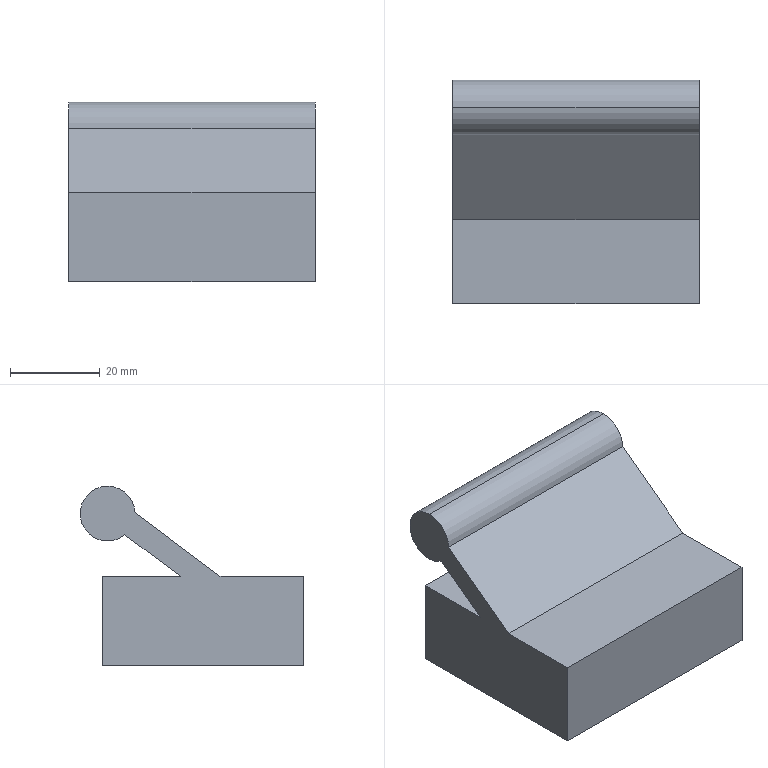Part | STEP file | Power switch 1 | 1 solid | 12 faces | box 55 x 49.883 x 40.112 mm | volume 61552 mm3 | plane 9 | cylinder 3 | commonest cylinder face diameters 12.241 x3
STEP:
#1=CARTESIAN_POINT('',(0.,0.,0.));
#2=DIRECTION('',(0.,0.,1.));
#3=DIRECTION('',(1.,0.,0.));
#4=AXIS2_PLACEMENT_3D('',#1,#2,#3);
#5=CARTESIAN_POINT('',(-27.5,21.263,27.872));
#6=VERTEX_POINT('',#5);
#7=CARTESIAN_POINT('',(-27.5,21.263,40.112));
#8=VERTEX_POINT('',#7);
#9=CARTESIAN_POINT('',(-27.5,21.263,33.992));
#10=DIRECTION('',(1.,0.,0.));
#11=DIRECTION('',(0.,0.,-1.));
#12=AXIS2_PLACEMENT_3D('',#9,#10,#11);
#13=CIRCLE('',#12,6.12);
#14=CARTESIAN_POINT('',(-27.5,21.263,33.992));
#15=DIRECTION('',(1.,0.,0.));
#16=DIRECTION('',(0.,0.,-1.));
#17=AXIS2_PLACEMENT_3D('',#14,#15,#16);
#18=CYLINDRICAL_SURFACE('',#17,6.12);
#19=CARTESIAN_POINT('',(0.,0.));
#20=DIRECTION('',(1.,0.));
#21=VECTOR('',#20,1.);
#22=LINE('',#19,#21);
#23=(GEOMETRIC_REPRESENTATION_CONTEXT(2)PARAMETRIC_REPRESENTATION_CONTEXT()REPRESENTATION_CONTEXT('',''));
#24=DEFINITIONAL_REPRESENTATION('',(#22),#23);
#25=PCURVE('',#18,#24);
#26=CARTESIAN_POINT('',(-27.5,22.5,20.));
#27=DIRECTION('',(1.,0.,0.));
#28=DIRECTION('',(0.,1.,0.));
#29=AXIS2_PLACEMENT_3D('',#26,#27,#28);
#30=PLANE('',#29);
#31=CARTESIAN_POINT('',(-1.237,13.992));
#32=DIRECTION('',(0.,-1.));
#33=AXIS2_PLACEMENT_2D('',#31,#32);
#34=CIRCLE('',#33,6.12);
#35=(GEOMETRIC_REPRESENTATION_CONTEXT(2)PARAMETRIC_REPRESENTATION_CONTEXT()REPRESENTATION_CONTEXT('',''));
#36=DEFINITIONAL_REPRESENTATION('',(#34),#35);
#37=PCURVE('',#30,#36);
#38=SURFACE_CURVE('',#13,(#25,#37),.PCURVE_S1.);
#39=EDGE_CURVE('',#6,#8,#38,.T.);
#40=ORIENTED_EDGE('',*,*,#39,.T.);
#41=CARTESIAN_POINT('',(27.5,21.263,40.112));
#42=VERTEX_POINT('',#41);
#43=CARTESIAN_POINT('',(-27.5,21.263,40.112));
#44=DIRECTION('',(1.,0.,0.));
#45=VECTOR('',#44,1.);
#46=LINE('',#43,#45);
#47=CARTESIAN_POINT('',(3.142,0.));
#48=DIRECTION('',(0.,1.));
#49=VECTOR('',#48,1.);
#50=LINE('',#47,#49);
#51=(GEOMETRIC_REPRESENTATION_CONTEXT(2)PARAMETRIC_REPRESENTATION_CONTEXT()REPRESENTATION_CONTEXT('',''));
#52=DEFINITIONAL_REPRESENTATION('',(#50),#51);
#53=PCURVE('',#18,#52);
#54=CARTESIAN_POINT('',(-27.5,21.263,33.992));
#55=DIRECTION('',(1.,0.,0.));
#56=DIRECTION('',(0.,0.,-1.));
#57=AXIS2_PLACEMENT_3D('',#54,#55,#56);
#58=CYLINDRICAL_SURFACE('',#57,6.12);
#59=CARTESIAN_POINT('',(3.142,0.));
#60=DIRECTION('',(0.,1.));
#61=VECTOR('',#60,1.);
#62=LINE('',#59,#61);
#63=(GEOMETRIC_REPRESENTATION_CONTEXT(2)PARAMETRIC_REPRESENTATION_CONTEXT()REPRESENTATION_CONTEXT('',''));
#64=DEFINITIONAL_REPRESENTATION('',(#62),#63);
#65=PCURVE('',#58,#64);
#66=SURFACE_CURVE('',#46,(#53,#65),.PCURVE_S1.);
#67=EDGE_CURVE('',#8,#42,#66,.T.);
#68=ORIENTED_EDGE('',*,*,#67,.T.);
#69=CARTESIAN_POINT('',(27.5,21.263,27.872));
#70=VERTEX_POINT('',#69);
#71=CARTESIAN_POINT('',(27.5,21.263,33.992));
#72=DIRECTION('',(-1.,0.,0.));
#73=DIRECTION('',(0.,0.,-1.));
#74=AXIS2_PLACEMENT_3D('',#71,#72,#73);
#75=CIRCLE('',#74,6.12);
#76=CARTESIAN_POINT('',(6.283,55.));
#77=DIRECTION('',(-1.,0.));
#78=VECTOR('',#77,1.);
#79=LINE('',#76,#78);
#80=(GEOMETRIC_REPRESENTATION_CONTEXT(2)PARAMETRIC_REPRESENTATION_CONTEXT()REPRESENTATION_CONTEXT('',''));
#81=DEFINITIONAL_REPRESENTATION('',(#79),#80);
#82=PCURVE('',#18,#81);
#83=CARTESIAN_POINT('',(27.5,22.5,20.));
#84=DIRECTION('',(-1.,0.,0.));
#85=DIRECTION('',(0.,-1.,0.));
#86=AXIS2_PLACEMENT_3D('',#83,#84,#85);
#87=PLANE('',#86);
#88=CARTESIAN_POINT('',(1.237,13.992));
#89=DIRECTION('',(0.,-1.));
#90=AXIS2_PLACEMENT_2D('',#88,#89);
#91=CIRCLE('',#90,6.12);
#92=(GEOMETRIC_REPRESENTATION_CONTEXT(2)PARAMETRIC_REPRESENTATION_CONTEXT()REPRESENTATION_CONTEXT('',''));
#93=DEFINITIONAL_REPRESENTATION('',(#91),#92);
#94=PCURVE('',#87,#93);
#95=SURFACE_CURVE('',#75,(#82,#94),.PCURVE_S1.);
#96=EDGE_CURVE('',#42,#70,#95,.T.);
#97=ORIENTED_EDGE('',*,*,#96,.T.);
#98=CARTESIAN_POINT('',(-27.5,21.263,27.872));
#99=DIRECTION('',(1.,0.,0.));
#100=VECTOR('',#99,1.);
#101=LINE('',#98,#100);
#102=CARTESIAN_POINT('',(0.,0.));
#103=DIRECTION('',(0.,1.));
#104=VECTOR('',#103,1.);
#105=LINE('',#102,#104);
#106=(GEOMETRIC_REPRESENTATION_CONTEXT(2)PARAMETRIC_REPRESENTATION_CONTEXT()REPRESENTATION_CONTEXT('',''));
#107=DEFINITIONAL_REPRESENTATION('',(#105),#106);
#108=PCURVE('',#18,#107);
#109=CARTESIAN_POINT('',(-27.5,21.263,33.992));
#110=DIRECTION('',(1.,0.,0.));
#111=DIRECTION('',(0.,0.,-1.));
#112=AXIS2_PLACEMENT_3D('',#109,#110,#111);
#113=CYLINDRICAL_SURFACE('',#112,6.12);
#114=CARTESIAN_POINT('',(6.283,0.));
#115=DIRECTION('',(0.,1.));
#116=VECTOR('',#115,1.);
#117=LINE('',#114,#116);
#118=(GEOMETRIC_REPRESENTATION_CONTEXT(2)PARAMETRIC_REPRESENTATION_CONTEXT()REPRESENTATION_CONTEXT('',''));
#119=DEFINITIONAL_REPRESENTATION('',(#117),#118);
#120=PCURVE('',#113,#119);
#121=SURFACE_CURVE('',#101,(#108,#120),.PCURVE_S1.);
#122=EDGE_CURVE('',#6,#70,#121,.T.);
#123=ORIENTED_EDGE('',*,*,#122,.F.);
#124=EDGE_LOOP('',(#40,#68,#97,#123));
#125=FACE_BOUND('',#124,.T.);
#126=ADVANCED_FACE('',(#125),#18,.T.);
#127=CARTESIAN_POINT('',(-27.5,17.412,29.235));
#128=VERTEX_POINT('',#127);
#129=CARTESIAN_POINT('',(-27.5,21.263,33.992));
#130=DIRECTION('',(1.,0.,0.));
#131=DIRECTION('',(0.,0.,-1.));
#132=AXIS2_PLACEMENT_3D('',#129,#130,#131);
#133=CIRCLE('',#132,6.12);
#134=CARTESIAN_POINT('',(0.,0.));
#135=DIRECTION('',(1.,0.));
#136=VECTOR('',#135,1.);
#137=LINE('',#134,#136);
#138=(GEOMETRIC_REPRESENTATION_CONTEXT(2)PARAMETRIC_REPRESENTATION_CONTEXT()REPRESENTATION_CONTEXT('',''));
#139=DEFINITIONAL_REPRESENTATION('',(#137),#138);
#140=PCURVE('',#113,#139);
#141=CARTESIAN_POINT('',(-1.237,13.992));
#142=DIRECTION('',(0.,-1.));
#143=AXIS2_PLACEMENT_2D('',#141,#142);
#144=CIRCLE('',#143,6.12);
#145=(GEOMETRIC_REPRESENTATION_CONTEXT(2)PARAMETRIC_REPRESENTATION_CONTEXT()REPRESENTATION_CONTEXT('',''));
#146=DEFINITIONAL_REPRESENTATION('',(#144),#145);
#147=PCURVE('',#30,#146);
#148=SURFACE_CURVE('',#133,(#140,#147),.PCURVE_S1.);
#149=EDGE_CURVE('',#128,#6,#148,.T.);
#150=ORIENTED_EDGE('',*,*,#149,.T.);
#151=ORIENTED_EDGE('',*,*,#122,.T.);
#152=CARTESIAN_POINT('',(27.5,17.412,29.235));
#153=VERTEX_POINT('',#152);
#154=CARTESIAN_POINT('',(27.5,21.263,33.992));
#155=DIRECTION('',(-1.,0.,0.));
#156=DIRECTION('',(0.,0.,-1.));
#157=AXIS2_PLACEMENT_3D('',#154,#155,#156);
#158=CIRCLE('',#157,6.12);
#159=CARTESIAN_POINT('',(6.283,55.));
#160=DIRECTION('',(-1.,0.));
#161=VECTOR('',#160,1.);
#162=LINE('',#159,#161);
#163=(GEOMETRIC_REPRESENTATION_CONTEXT(2)PARAMETRIC_REPRESENTATION_CONTEXT()REPRESENTATION_CONTEXT('',''));
#164=DEFINITIONAL_REPRESENTATION('',(#162),#163);
#165=PCURVE('',#113,#164);
#166=CARTESIAN_POINT('',(1.237,13.992));
#167=DIRECTION('',(0.,-1.));
#168=AXIS2_PLACEMENT_2D('',#166,#167);
#169=CIRCLE('',#168,6.12);
#170=(GEOMETRIC_REPRESENTATION_CONTEXT(2)PARAMETRIC_REPRESENTATION_CONTEXT()REPRESENTATION_CONTEXT('',''));
#171=DEFINITIONAL_REPRESENTATION('',(#169),#170);
#172=PCURVE('',#87,#171);
#173=SURFACE_CURVE('',#158,(#165,#172),.PCURVE_S1.);
#174=EDGE_CURVE('',#70,#153,#173,.T.);
#175=ORIENTED_EDGE('',*,*,#174,.T.);
#176=CARTESIAN_POINT('',(-27.5,17.412,29.235));
#177=DIRECTION('',(1.,0.,0.));
#178=VECTOR('',#177,1.);
#179=LINE('',#176,#178);
#180=CARTESIAN_POINT('',(5.603,0.));
#181=DIRECTION('',(0.,1.));
#182=VECTOR('',#181,1.);
#183=LINE('',#180,#182);
#184=(GEOMETRIC_REPRESENTATION_CONTEXT(2)PARAMETRIC_REPRESENTATION_CONTEXT()REPRESENTATION_CONTEXT('',''));
#185=DEFINITIONAL_REPRESENTATION('',(#183),#184);
#186=PCURVE('',#113,#185);
#187=CARTESIAN_POINT('',(-27.5,5.038,20.));
#188=DIRECTION('',(0.,0.5981,-0.8014));
#189=DIRECTION('',(0.,0.8014,0.5981));
#190=AXIS2_PLACEMENT_3D('',#187,#188,#189);
#191=PLANE('',#190);
#192=CARTESIAN_POINT('',(15.44,0.));
#193=DIRECTION('',(0.,1.));
#194=VECTOR('',#193,1.);
#195=LINE('',#192,#194);
#196=(GEOMETRIC_REPRESENTATION_CONTEXT(2)PARAMETRIC_REPRESENTATION_CONTEXT()REPRESENTATION_CONTEXT('',''));
#197=DEFINITIONAL_REPRESENTATION('',(#195),#196);
#198=PCURVE('',#191,#197);
#199=SURFACE_CURVE('',#179,(#186,#198),.PCURVE_S1.);
#200=EDGE_CURVE('',#128,#153,#199,.T.);
#201=ORIENTED_EDGE('',*,*,#200,.F.);
#202=EDGE_LOOP('',(#150,#151,#175,#201));
#203=FACE_BOUND('',#202,.T.);
#204=ADVANCED_FACE('',(#203),#113,.T.);
#205=CARTESIAN_POINT('',(-27.5,-22.5,0.));
#206=VERTEX_POINT('',#205);
#207=CARTESIAN_POINT('',(27.5,-22.5,0.));
#208=VERTEX_POINT('',#207);
#209=CARTESIAN_POINT('',(27.5,-22.5,0.));
#210=DIRECTION('',(1.,0.,0.));
#211=VECTOR('',#210,1.);
#212=LINE('',#209,#211);
#213=CARTESIAN_POINT('',(27.5,-22.5,0.));
#214=DIRECTION('',(0.,0.,1.));
#215=DIRECTION('',(1.,0.,0.));
#216=AXIS2_PLACEMENT_3D('',#213,#214,#215);
#217=PLANE('',#216);
#218=CARTESIAN_POINT('',(0.,0.));
#219=DIRECTION('',(1.,0.));
#220=VECTOR('',#219,1.);
#221=LINE('',#218,#220);
#222=(GEOMETRIC_REPRESENTATION_CONTEXT(2)PARAMETRIC_REPRESENTATION_CONTEXT()REPRESENTATION_CONTEXT('',''));
#223=DEFINITIONAL_REPRESENTATION('',(#221),#222);
#224=PCURVE('',#217,#223);
#225=CARTESIAN_POINT('',(-27.5,-22.5,20.));
#226=DIRECTION('',(0.,1.,0.));
#227=DIRECTION('',(0.,0.,1.));
#228=AXIS2_PLACEMENT_3D('',#225,#226,#227);
#229=PLANE('',#228);
#230=CARTESIAN_POINT('',(-20.,55.));
#231=DIRECTION('',(0.,1.));
#232=VECTOR('',#231,1.);
#233=LINE('',#230,#232);
#234=(GEOMETRIC_REPRESENTATION_CONTEXT(2)PARAMETRIC_REPRESENTATION_CONTEXT()REPRESENTATION_CONTEXT('',''));
#235=DEFINITIONAL_REPRESENTATION('',(#233),#234);
#236=PCURVE('',#229,#235);
#237=SURFACE_CURVE('',#212,(#224,#236),.PCURVE_S1.);
#238=EDGE_CURVE('',#206,#208,#237,.T.);
#239=ORIENTED_EDGE('',*,*,#238,.F.);
#240=CARTESIAN_POINT('',(-27.5,22.5,0.));
#241=VERTEX_POINT('',#240);
#242=CARTESIAN_POINT('',(-27.5,-22.5,0.));
#243=DIRECTION('',(0.,-1.,0.));
#244=VECTOR('',#243,1.);
#245=LINE('',#242,#244);
#246=CARTESIAN_POINT('',(-55.,0.));
#247=DIRECTION('',(0.,-1.));
#248=VECTOR('',#247,1.);
#249=LINE('',#246,#248);
#250=(GEOMETRIC_REPRESENTATION_CONTEXT(2)PARAMETRIC_REPRESENTATION_CONTEXT()REPRESENTATION_CONTEXT('',''));
#251=DEFINITIONAL_REPRESENTATION('',(#249),#250);
#252=PCURVE('',#217,#251);
#253=CARTESIAN_POINT('',(-45.,-20.));
#254=DIRECTION('',(-1.,0.));
#255=VECTOR('',#254,1.);
#256=LINE('',#253,#255);
#257=(GEOMETRIC_REPRESENTATION_CONTEXT(2)PARAMETRIC_REPRESENTATION_CONTEXT()REPRESENTATION_CONTEXT('',''));
#258=DEFINITIONAL_REPRESENTATION('',(#256),#257);
#259=PCURVE('',#30,#258);
#260=SURFACE_CURVE('',#245,(#252,#259),.PCURVE_S1.);
#261=EDGE_CURVE('',#241,#206,#260,.T.);
#262=ORIENTED_EDGE('',*,*,#261,.F.);
#263=CARTESIAN_POINT('',(27.5,22.5,0.));
#264=VERTEX_POINT('',#263);
#265=CARTESIAN_POINT('',(27.5,22.5,0.));
#266=DIRECTION('',(-1.,0.,0.));
#267=VECTOR('',#266,1.);
#268=LINE('',#265,#267);
#269=CARTESIAN_POINT('',(0.,45.));
#270=DIRECTION('',(-1.,0.));
#271=VECTOR('',#270,1.);
#272=LINE('',#269,#271);
#273=(GEOMETRIC_REPRESENTATION_CONTEXT(2)PARAMETRIC_REPRESENTATION_CONTEXT()REPRESENTATION_CONTEXT('',''));
#274=DEFINITIONAL_REPRESENTATION('',(#272),#273);
#275=PCURVE('',#217,#274);
#276=CARTESIAN_POINT('',(-27.5,22.5,20.));
#277=DIRECTION('',(0.,-1.,0.));
#278=DIRECTION('',(0.,0.,-1.));
#279=AXIS2_PLACEMENT_3D('',#276,#277,#278);
#280=PLANE('',#279);
#281=CARTESIAN_POINT('',(20.,55.));
#282=DIRECTION('',(0.,-1.));
#283=VECTOR('',#282,1.);
#284=LINE('',#281,#283);
#285=(GEOMETRIC_REPRESENTATION_CONTEXT(2)PARAMETRIC_REPRESENTATION_CONTEXT()REPRESENTATION_CONTEXT('',''));
#286=DEFINITIONAL_REPRESENTATION('',(#284),#285);
#287=PCURVE('',#280,#286);
#288=SURFACE_CURVE('',#268,(#275,#287),.PCURVE_S1.);
#289=EDGE_CURVE('',#264,#241,#288,.T.);
#290=ORIENTED_EDGE('',*,*,#289,.F.);
#291=CARTESIAN_POINT('',(27.5,-22.5,0.));
#292=DIRECTION('',(0.,1.,0.));
#293=VECTOR('',#292,1.);
#294=LINE('',#291,#293);
#295=CARTESIAN_POINT('',(0.,0.));
#296=DIRECTION('',(0.,1.));
#297=VECTOR('',#296,1.);
#298=LINE('',#295,#297);
#299=(GEOMETRIC_REPRESENTATION_CONTEXT(2)PARAMETRIC_REPRESENTATION_CONTEXT()REPRESENTATION_CONTEXT('',''));
#300=DEFINITIONAL_REPRESENTATION('',(#298),#299);
#301=PCURVE('',#217,#300);
#302=CARTESIAN_POINT('',(45.,-20.));
#303=DIRECTION('',(-1.,0.));
#304=VECTOR('',#303,1.);
#305=LINE('',#302,#304);
#306=(GEOMETRIC_REPRESENTATION_CONTEXT(2)PARAMETRIC_REPRESENTATION_CONTEXT()REPRESENTATION_CONTEXT('',''));
#307=DEFINITIONAL_REPRESENTATION('',(#305),#306);
#308=PCURVE('',#87,#307);
#309=SURFACE_CURVE('',#294,(#301,#308),.PCURVE_S1.);
#310=EDGE_CURVE('',#208,#264,#309,.T.);
#311=ORIENTED_EDGE('',*,*,#310,.F.);
#312=EDGE_LOOP('',(#239,#262,#290,#311));
#313=FACE_BOUND('',#312,.T.);
#314=ADVANCED_FACE('',(#313),#217,.F.);
#315=CARTESIAN_POINT('',(27.5,22.5,20.));
#316=VERTEX_POINT('',#315);
#317=CARTESIAN_POINT('',(27.5,22.5,20.));
#318=DIRECTION('',(0.,0.,-1.));
#319=VECTOR('',#318,1.);
#320=LINE('',#317,#319);
#321=CARTESIAN_POINT('',(0.,0.));
#322=DIRECTION('',(0.,-1.));
#323=VECTOR('',#322,1.);
#324=LINE('',#321,#323);
#325=(GEOMETRIC_REPRESENTATION_CONTEXT(2)PARAMETRIC_REPRESENTATION_CONTEXT()REPRESENTATION_CONTEXT('',''));
#326=DEFINITIONAL_REPRESENTATION('',(#324),#325);
#327=PCURVE('',#87,#326);
#328=CARTESIAN_POINT('',(0.,55.));
#329=DIRECTION('',(1.,0.));
#330=VECTOR('',#329,1.);
#331=LINE('',#328,#330);
#332=(GEOMETRIC_REPRESENTATION_CONTEXT(2)PARAMETRIC_REPRESENTATION_CONTEXT()REPRESENTATION_CONTEXT('',''));
#333=DEFINITIONAL_REPRESENTATION('',(#331),#332);
#334=PCURVE('',#280,#333);
#335=SURFACE_CURVE('',#320,(#327,#334),.PCURVE_S1.);
#336=EDGE_CURVE('',#316,#264,#335,.T.);
#337=ORIENTED_EDGE('',*,*,#336,.F.);
#338=CARTESIAN_POINT('',(27.5,5.038,20.));
#339=VERTEX_POINT('',#338);
#340=CARTESIAN_POINT('',(27.5,22.5,20.));
#341=DIRECTION('',(0.,1.,0.));
#342=VECTOR('',#341,1.);
#343=LINE('',#340,#342);
#344=CARTESIAN_POINT('',(0.,0.));
#345=DIRECTION('',(-1.,0.));
#346=VECTOR('',#345,1.);
#347=LINE('',#344,#346);
#348=(GEOMETRIC_REPRESENTATION_CONTEXT(2)PARAMETRIC_REPRESENTATION_CONTEXT()REPRESENTATION_CONTEXT('',''));
#349=DEFINITIONAL_REPRESENTATION('',(#347),#348);
#350=PCURVE('',#87,#349);
#351=CARTESIAN_POINT('',(27.5,-22.5,20.));
#352=DIRECTION('',(0.,0.,1.));
#353=DIRECTION('',(1.,0.,0.));
#354=AXIS2_PLACEMENT_3D('',#351,#352,#353);
#355=PLANE('',#354);
#356=CARTESIAN_POINT('',(0.,45.));
#357=DIRECTION('',(0.,1.));
#358=VECTOR('',#357,1.);
#359=LINE('',#356,#358);
#360=(GEOMETRIC_REPRESENTATION_CONTEXT(2)PARAMETRIC_REPRESENTATION_CONTEXT()REPRESENTATION_CONTEXT('',''));
#361=DEFINITIONAL_REPRESENTATION('',(#359),#360);
#362=PCURVE('',#355,#361);
#363=SURFACE_CURVE('',#343,(#350,#362),.PCURVE_S1.);
#364=EDGE_CURVE('',#339,#316,#363,.T.);
#365=ORIENTED_EDGE('',*,*,#364,.F.);
#366=CARTESIAN_POINT('',(27.5,17.412,29.235));
#367=DIRECTION('',(0.,-0.8014,-0.5981));
#368=VECTOR('',#367,1.);
#369=LINE('',#366,#368);
#370=CARTESIAN_POINT('',(5.088,9.235));
#371=DIRECTION('',(0.8014,-0.5981));
#372=VECTOR('',#371,1.);
#373=LINE('',#370,#372);
#374=(GEOMETRIC_REPRESENTATION_CONTEXT(2)PARAMETRIC_REPRESENTATION_CONTEXT()REPRESENTATION_CONTEXT('',''));
#375=DEFINITIONAL_REPRESENTATION('',(#373),#374);
#376=PCURVE('',#87,#375);
#377=CARTESIAN_POINT('',(15.44,55.));
#378=DIRECTION('',(-1.,0.));
#379=VECTOR('',#378,1.);
#380=LINE('',#377,#379);
#381=(GEOMETRIC_REPRESENTATION_CONTEXT(2)PARAMETRIC_REPRESENTATION_CONTEXT()REPRESENTATION_CONTEXT('',''));
#382=DEFINITIONAL_REPRESENTATION('',(#380),#381);
#383=PCURVE('',#191,#382);
#384=SURFACE_CURVE('',#369,(#376,#383),.PCURVE_S1.);
#385=EDGE_CURVE('',#153,#339,#384,.T.);
#386=ORIENTED_EDGE('',*,*,#385,.F.);
#387=ORIENTED_EDGE('',*,*,#174,.F.);
#388=ORIENTED_EDGE('',*,*,#96,.F.);
#389=CARTESIAN_POINT('',(27.5,15.145,34.163));
#390=VERTEX_POINT('',#389);
#391=CARTESIAN_POINT('',(27.5,21.263,33.992));
#392=DIRECTION('',(-1.,0.,0.));
#393=DIRECTION('',(0.,0.,-1.));
#394=AXIS2_PLACEMENT_3D('',#391,#392,#393);
#395=CIRCLE('',#394,6.12);
#396=CARTESIAN_POINT('',(1.237,13.992));
#397=DIRECTION('',(0.,-1.));
#398=AXIS2_PLACEMENT_2D('',#396,#397);
#399=CIRCLE('',#398,6.12);
#400=(GEOMETRIC_REPRESENTATION_CONTEXT(2)PARAMETRIC_REPRESENTATION_CONTEXT()REPRESENTATION_CONTEXT('',''));
#401=DEFINITIONAL_REPRESENTATION('',(#399),#400);
#402=PCURVE('',#87,#401);
#403=CARTESIAN_POINT('',(6.283,55.));
#404=DIRECTION('',(-1.,0.));
#405=VECTOR('',#404,1.);
#406=LINE('',#403,#405);
#407=(GEOMETRIC_REPRESENTATION_CONTEXT(2)PARAMETRIC_REPRESENTATION_CONTEXT()REPRESENTATION_CONTEXT('',''));
#408=DEFINITIONAL_REPRESENTATION('',(#406),#407);
#409=PCURVE('',#58,#408);
#410=SURFACE_CURVE('',#395,(#402,#409),.PCURVE_S1.);
#411=EDGE_CURVE('',#390,#42,#410,.T.);
#412=ORIENTED_EDGE('',*,*,#411,.F.);
#413=CARTESIAN_POINT('',(27.5,-3.831,20.));
#414=VERTEX_POINT('',#413);
#415=CARTESIAN_POINT('',(27.5,-3.831,20.));
#416=DIRECTION('',(0.,0.8014,0.5981));
#417=VECTOR('',#416,1.);
#418=LINE('',#415,#417);
#419=CARTESIAN_POINT('',(26.331,0.));
#420=DIRECTION('',(-0.8014,0.5981));
#421=VECTOR('',#420,1.);
#422=LINE('',#419,#421);
#423=(GEOMETRIC_REPRESENTATION_CONTEXT(2)PARAMETRIC_REPRESENTATION_CONTEXT()REPRESENTATION_CONTEXT('',''));
#424=DEFINITIONAL_REPRESENTATION('',(#422),#423);
#425=PCURVE('',#87,#424);
#426=CARTESIAN_POINT('',(-27.5,15.145,34.163));
#427=DIRECTION('',(0.,-0.5981,0.8014));
#428=DIRECTION('',(0.,-0.8014,-0.5981));
#429=AXIS2_PLACEMENT_3D('',#426,#427,#428);
#430=PLANE('',#429);
#431=CARTESIAN_POINT('',(23.679,55.));
#432=DIRECTION('',(-1.,0.));
#433=VECTOR('',#432,1.);
#434=LINE('',#431,#433);
#435=(GEOMETRIC_REPRESENTATION_CONTEXT(2)PARAMETRIC_REPRESENTATION_CONTEXT()REPRESENTATION_CONTEXT('',''));
#436=DEFINITIONAL_REPRESENTATION('',(#434),#435);
#437=PCURVE('',#430,#436);
#438=SURFACE_CURVE('',#418,(#425,#437),.PCURVE_S1.);
#439=EDGE_CURVE('',#414,#390,#438,.T.);
#440=ORIENTED_EDGE('',*,*,#439,.F.);
#441=CARTESIAN_POINT('',(27.5,-22.5,20.));
#442=VERTEX_POINT('',#441);
#443=CARTESIAN_POINT('',(27.5,22.5,20.));
#444=DIRECTION('',(0.,1.,0.));
#445=VECTOR('',#444,1.);
#446=LINE('',#443,#445);
#447=CARTESIAN_POINT('',(0.,0.));
#448=DIRECTION('',(-1.,0.));
#449=VECTOR('',#448,1.);
#450=LINE('',#447,#449);
#451=(GEOMETRIC_REPRESENTATION_CONTEXT(2)PARAMETRIC_REPRESENTATION_CONTEXT()REPRESENTATION_CONTEXT('',''));
#452=DEFINITIONAL_REPRESENTATION('',(#450),#451);
#453=PCURVE('',#87,#452);
#454=CARTESIAN_POINT('',(27.5,-22.5,20.));
#455=DIRECTION('',(0.,0.,1.));
#456=DIRECTION('',(1.,0.,0.));
#457=AXIS2_PLACEMENT_3D('',#454,#455,#456);
#458=PLANE('',#457);
#459=CARTESIAN_POINT('',(0.,45.));
#460=DIRECTION('',(0.,1.));
#461=VECTOR('',#460,1.);
#462=LINE('',#459,#461);
#463=(GEOMETRIC_REPRESENTATION_CONTEXT(2)PARAMETRIC_REPRESENTATION_CONTEXT()REPRESENTATION_CONTEXT('',''));
#464=DEFINITIONAL_REPRESENTATION('',(#462),#463);
#465=PCURVE('',#458,#464);
#466=SURFACE_CURVE('',#446,(#453,#465),.PCURVE_S1.);
#467=EDGE_CURVE('',#442,#414,#466,.T.);
#468=ORIENTED_EDGE('',*,*,#467,.F.);
#469=CARTESIAN_POINT('',(27.5,-22.5,20.));
#470=DIRECTION('',(0.,0.,1.));
#471=VECTOR('',#470,1.);
#472=LINE('',#469,#471);
#473=CARTESIAN_POINT('',(45.,0.));
#474=DIRECTION('',(0.,1.));
#475=VECTOR('',#474,1.);
#476=LINE('',#473,#475);
#477=(GEOMETRIC_REPRESENTATION_CONTEXT(2)PARAMETRIC_REPRESENTATION_CONTEXT()REPRESENTATION_CONTEXT('',''));
#478=DEFINITIONAL_REPRESENTATION('',(#476),#477);
#479=PCURVE('',#87,#478);
#480=CARTESIAN_POINT('',(0.,55.));
#481=DIRECTION('',(1.,0.));
#482=VECTOR('',#481,1.);
#483=LINE('',#480,#482);
#484=(GEOMETRIC_REPRESENTATION_CONTEXT(2)PARAMETRIC_REPRESENTATION_CONTEXT()REPRESENTATION_CONTEXT('',''));
#485=DEFINITIONAL_REPRESENTATION('',(#483),#484);
#486=PCURVE('',#229,#485);
#487=SURFACE_CURVE('',#472,(#479,#486),.PCURVE_S1.);
#488=EDGE_CURVE('',#208,#442,#487,.T.);
#489=ORIENTED_EDGE('',*,*,#488,.F.);
#490=ORIENTED_EDGE('',*,*,#310,.T.);
#491=EDGE_LOOP('',(#337,#365,#386,#387,#388,#412,#440,#468,#489,#490));
#492=FACE_BOUND('',#491,.T.);
#493=ADVANCED_FACE('',(#492),#87,.F.);
#494=ORIENTED_EDGE('',*,*,#488,.T.);
#495=CARTESIAN_POINT('',(-27.5,-22.5,20.));
#496=VERTEX_POINT('',#495);
#497=CARTESIAN_POINT('',(-27.5,-22.5,20.));
#498=DIRECTION('',(1.,0.,0.));
#499=VECTOR('',#498,1.);
#500=LINE('',#497,#499);
#501=CARTESIAN_POINT('',(0.,0.));
#502=DIRECTION('',(0.,1.));
#503=VECTOR('',#502,1.);
#504=LINE('',#501,#503);
#505=(GEOMETRIC_REPRESENTATION_CONTEXT(2)PARAMETRIC_REPRESENTATION_CONTEXT()REPRESENTATION_CONTEXT('',''));
#506=DEFINITIONAL_REPRESENTATION('',(#504),#505);
#507=PCURVE('',#229,#506);
#508=CARTESIAN_POINT('',(-55.,0.));
#509=DIRECTION('',(1.,0.));
#510=VECTOR('',#509,1.);
#511=LINE('',#508,#510);
#512=(GEOMETRIC_REPRESENTATION_CONTEXT(2)PARAMETRIC_REPRESENTATION_CONTEXT()REPRESENTATION_CONTEXT('',''));
#513=DEFINITIONAL_REPRESENTATION('',(#511),#512);
#514=PCURVE('',#458,#513);
#515=SURFACE_CURVE('',#500,(#507,#514),.PCURVE_S1.);
#516=EDGE_CURVE('',#496,#442,#515,.T.);
#517=ORIENTED_EDGE('',*,*,#516,.F.);
#518=CARTESIAN_POINT('',(-27.5,-22.5,20.));
#519=DIRECTION('',(0.,0.,1.));
#520=VECTOR('',#519,1.);
#521=LINE('',#518,#520);
#522=CARTESIAN_POINT('',(0.,0.));
#523=DIRECTION('',(1.,0.));
#524=VECTOR('',#523,1.);
#525=LINE('',#522,#524);
#526=(GEOMETRIC_REPRESENTATION_CONTEXT(2)PARAMETRIC_REPRESENTATION_CONTEXT()REPRESENTATION_CONTEXT('',''));
#527=DEFINITIONAL_REPRESENTATION('',(#525),#526);
#528=PCURVE('',#229,#527);
#529=CARTESIAN_POINT('',(-45.,0.));
#530=DIRECTION('',(0.,1.));
#531=VECTOR('',#530,1.);
#532=LINE('',#529,#531);
#533=(GEOMETRIC_REPRESENTATION_CONTEXT(2)PARAMETRIC_REPRESENTATION_CONTEXT()REPRESENTATION_CONTEXT('',''));
#534=DEFINITIONAL_REPRESENTATION('',(#532),#533);
#535=PCURVE('',#30,#534);
#536=SURFACE_CURVE('',#521,(#528,#535),.PCURVE_S1.);
#537=EDGE_CURVE('',#206,#496,#536,.T.);
#538=ORIENTED_EDGE('',*,*,#537,.F.);
#539=ORIENTED_EDGE('',*,*,#238,.T.);
#540=EDGE_LOOP('',(#494,#517,#538,#539));
#541=FACE_BOUND('',#540,.T.);
#542=ADVANCED_FACE('',(#541),#229,.F.);
#543=ORIENTED_EDGE('',*,*,#537,.T.);
#544=CARTESIAN_POINT('',(-27.5,-3.831,20.));
#545=VERTEX_POINT('',#544);
#546=CARTESIAN_POINT('',(-27.5,22.5,20.));
#547=DIRECTION('',(0.,-1.,0.));
#548=VECTOR('',#547,1.);
#549=LINE('',#546,#548);
#550=CARTESIAN_POINT('',(0.,0.));
#551=DIRECTION('',(-1.,0.));
#552=VECTOR('',#551,1.);
#553=LINE('',#550,#552);
#554=(GEOMETRIC_REPRESENTATION_CONTEXT(2)PARAMETRIC_REPRESENTATION_CONTEXT()REPRESENTATION_CONTEXT('',''));
#555=DEFINITIONAL_REPRESENTATION('',(#553),#554);
#556=PCURVE('',#30,#555);
#557=CARTESIAN_POINT('',(-55.,45.));
#558=DIRECTION('',(0.,-1.));
#559=VECTOR('',#558,1.);
#560=LINE('',#557,#559);
#561=(GEOMETRIC_REPRESENTATION_CONTEXT(2)PARAMETRIC_REPRESENTATION_CONTEXT()REPRESENTATION_CONTEXT('',''));
#562=DEFINITIONAL_REPRESENTATION('',(#560),#561);
#563=PCURVE('',#458,#562);
#564=SURFACE_CURVE('',#549,(#556,#563),.PCURVE_S1.);
#565=EDGE_CURVE('',#545,#496,#564,.T.);
#566=ORIENTED_EDGE('',*,*,#565,.F.);
#567=CARTESIAN_POINT('',(-27.5,15.145,34.163));
#568=VERTEX_POINT('',#567);
#569=CARTESIAN_POINT('',(-27.5,15.145,34.163));
#570=DIRECTION('',(0.,-0.8014,-0.5981));
#571=VECTOR('',#570,1.);
#572=LINE('',#569,#571);
#573=CARTESIAN_POINT('',(-7.355,14.163));
#574=DIRECTION('',(-0.8014,-0.5981));
#575=VECTOR('',#574,1.);
#576=LINE('',#573,#575);
#577=(GEOMETRIC_REPRESENTATION_CONTEXT(2)PARAMETRIC_REPRESENTATION_CONTEXT()REPRESENTATION_CONTEXT('',''));
#578=DEFINITIONAL_REPRESENTATION('',(#576),#577);
#579=PCURVE('',#30,#578);
#580=CARTESIAN_POINT('',(0.,0.));
#581=DIRECTION('',(1.,0.));
#582=VECTOR('',#581,1.);
#583=LINE('',#580,#582);
#584=(GEOMETRIC_REPRESENTATION_CONTEXT(2)PARAMETRIC_REPRESENTATION_CONTEXT()REPRESENTATION_CONTEXT('',''));
#585=DEFINITIONAL_REPRESENTATION('',(#583),#584);
#586=PCURVE('',#430,#585);
#587=SURFACE_CURVE('',#572,(#579,#586),.PCURVE_S1.);
#588=EDGE_CURVE('',#568,#545,#587,.T.);
#589=ORIENTED_EDGE('',*,*,#588,.F.);
#590=CARTESIAN_POINT('',(-27.5,21.263,33.992));
#591=DIRECTION('',(1.,0.,0.));
#592=DIRECTION('',(0.,0.,-1.));
#593=AXIS2_PLACEMENT_3D('',#590,#591,#592);
#594=CIRCLE('',#593,6.12);
#595=CARTESIAN_POINT('',(-1.237,13.992));
#596=DIRECTION('',(0.,-1.));
#597=AXIS2_PLACEMENT_2D('',#595,#596);
#598=CIRCLE('',#597,6.12);
#599=(GEOMETRIC_REPRESENTATION_CONTEXT(2)PARAMETRIC_REPRESENTATION_CONTEXT()REPRESENTATION_CONTEXT('',''));
#600=DEFINITIONAL_REPRESENTATION('',(#598),#599);
#601=PCURVE('',#30,#600);
#602=CARTESIAN_POINT('',(0.,0.));
#603=DIRECTION('',(1.,0.));
#604=VECTOR('',#603,1.);
#605=LINE('',#602,#604);
#606=(GEOMETRIC_REPRESENTATION_CONTEXT(2)PARAMETRIC_REPRESENTATION_CONTEXT()REPRESENTATION_CONTEXT('',''));
#607=DEFINITIONAL_REPRESENTATION('',(#605),#606);
#608=PCURVE('',#58,#607);
#609=SURFACE_CURVE('',#594,(#601,#608),.PCURVE_S1.);
#610=EDGE_CURVE('',#8,#568,#609,.T.);
#611=ORIENTED_EDGE('',*,*,#610,.F.);
#612=ORIENTED_EDGE('',*,*,#39,.F.);
#613=ORIENTED_EDGE('',*,*,#149,.F.);
#614=CARTESIAN_POINT('',(-27.5,5.038,20.));
#615=VERTEX_POINT('',#614);
#616=CARTESIAN_POINT('',(-27.5,5.038,20.));
#617=DIRECTION('',(0.,0.8014,0.5981));
#618=VECTOR('',#617,1.);
#619=LINE('',#616,#618);
#620=CARTESIAN_POINT('',(-17.462,0.));
#621=DIRECTION('',(0.8014,0.5981));
#622=VECTOR('',#621,1.);
#623=LINE('',#620,#622);
#624=(GEOMETRIC_REPRESENTATION_CONTEXT(2)PARAMETRIC_REPRESENTATION_CONTEXT()REPRESENTATION_CONTEXT('',''));
#625=DEFINITIONAL_REPRESENTATION('',(#623),#624);
#626=PCURVE('',#30,#625);
#627=CARTESIAN_POINT('',(0.,0.));
#628=DIRECTION('',(1.,0.));
#629=VECTOR('',#628,1.);
#630=LINE('',#627,#629);
#631=(GEOMETRIC_REPRESENTATION_CONTEXT(2)PARAMETRIC_REPRESENTATION_CONTEXT()REPRESENTATION_CONTEXT('',''));
#632=DEFINITIONAL_REPRESENTATION('',(#630),#631);
#633=PCURVE('',#191,#632);
#634=SURFACE_CURVE('',#619,(#626,#633),.PCURVE_S1.);
#635=EDGE_CURVE('',#615,#128,#634,.T.);
#636=ORIENTED_EDGE('',*,*,#635,.F.);
#637=CARTESIAN_POINT('',(-27.5,22.5,20.));
#638=VERTEX_POINT('',#637);
#639=CARTESIAN_POINT('',(-27.5,22.5,20.));
#640=DIRECTION('',(0.,-1.,0.));
#641=VECTOR('',#640,1.);
#642=LINE('',#639,#641);
#643=CARTESIAN_POINT('',(0.,0.));
#644=DIRECTION('',(-1.,0.));
#645=VECTOR('',#644,1.);
#646=LINE('',#643,#645);
#647=(GEOMETRIC_REPRESENTATION_CONTEXT(2)PARAMETRIC_REPRESENTATION_CONTEXT()REPRESENTATION_CONTEXT('',''));
#648=DEFINITIONAL_REPRESENTATION('',(#646),#647);
#649=PCURVE('',#30,#648);
#650=CARTESIAN_POINT('',(-55.,45.));
#651=DIRECTION('',(0.,-1.));
#652=VECTOR('',#651,1.);
#653=LINE('',#650,#652);
#654=(GEOMETRIC_REPRESENTATION_CONTEXT(2)PARAMETRIC_REPRESENTATION_CONTEXT()REPRESENTATION_CONTEXT('',''));
#655=DEFINITIONAL_REPRESENTATION('',(#653),#654);
#656=PCURVE('',#355,#655);
#657=SURFACE_CURVE('',#642,(#649,#656),.PCURVE_S1.);
#658=EDGE_CURVE('',#638,#615,#657,.T.);
#659=ORIENTED_EDGE('',*,*,#658,.F.);
#660=CARTESIAN_POINT('',(-27.5,22.5,20.));
#661=DIRECTION('',(0.,0.,1.));
#662=VECTOR('',#661,1.);
#663=LINE('',#660,#662);
#664=CARTESIAN_POINT('',(0.,0.));
#665=DIRECTION('',(0.,1.));
#666=VECTOR('',#665,1.);
#667=LINE('',#664,#666);
#668=(GEOMETRIC_REPRESENTATION_CONTEXT(2)PARAMETRIC_REPRESENTATION_CONTEXT()REPRESENTATION_CONTEXT('',''));
#669=DEFINITIONAL_REPRESENTATION('',(#667),#668);
#670=PCURVE('',#30,#669);
#671=CARTESIAN_POINT('',(0.,0.));
#672=DIRECTION('',(-1.,0.));
#673=VECTOR('',#672,1.);
#674=LINE('',#671,#673);
#675=(GEOMETRIC_REPRESENTATION_CONTEXT(2)PARAMETRIC_REPRESENTATION_CONTEXT()REPRESENTATION_CONTEXT('',''));
#676=DEFINITIONAL_REPRESENTATION('',(#674),#675);
#677=PCURVE('',#280,#676);
#678=SURFACE_CURVE('',#663,(#670,#677),.PCURVE_S1.);
#679=EDGE_CURVE('',#241,#638,#678,.T.);
#680=ORIENTED_EDGE('',*,*,#679,.F.);
#681=ORIENTED_EDGE('',*,*,#261,.T.);
#682=EDGE_LOOP('',(#543,#566,#589,#611,#612,#613,#636,#659,#680,#681));
#683=FACE_BOUND('',#682,.T.);
#684=ADVANCED_FACE('',(#683),#30,.F.);
#685=ORIENTED_EDGE('',*,*,#679,.T.);
#686=CARTESIAN_POINT('',(-27.5,22.5,20.));
#687=DIRECTION('',(-1.,0.,0.));
#688=VECTOR('',#687,1.);
#689=LINE('',#686,#688);
#690=CARTESIAN_POINT('',(0.,0.));
#691=DIRECTION('',(0.,-1.));
#692=VECTOR('',#691,1.);
#693=LINE('',#690,#692);
#694=(GEOMETRIC_REPRESENTATION_CONTEXT(2)PARAMETRIC_REPRESENTATION_CONTEXT()REPRESENTATION_CONTEXT('',''));
#695=DEFINITIONAL_REPRESENTATION('',(#693),#694);
#696=PCURVE('',#280,#695);
#697=CARTESIAN_POINT('',(-55.,45.));
#698=DIRECTION('',(-1.,0.));
#699=VECTOR('',#698,1.);
#700=LINE('',#697,#699);
#701=(GEOMETRIC_REPRESENTATION_CONTEXT(2)PARAMETRIC_REPRESENTATION_CONTEXT()REPRESENTATION_CONTEXT('',''));
#702=DEFINITIONAL_REPRESENTATION('',(#700),#701);
#703=PCURVE('',#355,#702);
#704=SURFACE_CURVE('',#689,(#696,#703),.PCURVE_S1.);
#705=EDGE_CURVE('',#316,#638,#704,.T.);
#706=ORIENTED_EDGE('',*,*,#705,.F.);
#707=ORIENTED_EDGE('',*,*,#336,.T.);
#708=ORIENTED_EDGE('',*,*,#289,.T.);
#709=EDGE_LOOP('',(#685,#706,#707,#708));
#710=FACE_BOUND('',#709,.T.);
#711=ADVANCED_FACE('',(#710),#280,.F.);
#712=ORIENTED_EDGE('',*,*,#364,.T.);
#713=ORIENTED_EDGE('',*,*,#705,.T.);
#714=ORIENTED_EDGE('',*,*,#658,.T.);
#715=CARTESIAN_POINT('',(27.5,5.038,20.));
#716=DIRECTION('',(1.,0.,0.));
#717=VECTOR('',#716,1.);
#718=LINE('',#715,#717);
#719=CARTESIAN_POINT('',(0.,27.538));
#720=DIRECTION('',(1.,0.));
#721=VECTOR('',#720,1.);
#722=LINE('',#719,#721);
#723=(GEOMETRIC_REPRESENTATION_CONTEXT(2)PARAMETRIC_REPRESENTATION_CONTEXT()REPRESENTATION_CONTEXT('',''));
#724=DEFINITIONAL_REPRESENTATION('',(#722),#723);
#725=PCURVE('',#355,#724);
#726=CARTESIAN_POINT('',(0.,55.));
#727=DIRECTION('',(0.,1.));
#728=VECTOR('',#727,1.);
#729=LINE('',#726,#728);
#730=(GEOMETRIC_REPRESENTATION_CONTEXT(2)PARAMETRIC_REPRESENTATION_CONTEXT()REPRESENTATION_CONTEXT('',''));
#731=DEFINITIONAL_REPRESENTATION('',(#729),#730);
#732=PCURVE('',#191,#731);
#733=SURFACE_CURVE('',#718,(#725,#732),.PCURVE_S1.);
#734=EDGE_CURVE('',#615,#339,#733,.T.);
#735=ORIENTED_EDGE('',*,*,#734,.T.);
#736=EDGE_LOOP('',(#712,#713,#714,#735));
#737=FACE_BOUND('',#736,.T.);
#738=ADVANCED_FACE('',(#737),#355,.T.);
#739=ORIENTED_EDGE('',*,*,#635,.T.);
#740=ORIENTED_EDGE('',*,*,#200,.T.);
#741=ORIENTED_EDGE('',*,*,#385,.T.);
#742=ORIENTED_EDGE('',*,*,#734,.F.);
#743=EDGE_LOOP('',(#739,#740,#741,#742));
#744=FACE_BOUND('',#743,.T.);
#745=ADVANCED_FACE('',(#744),#191,.T.);
#746=ORIENTED_EDGE('',*,*,#67,.F.);
#747=ORIENTED_EDGE('',*,*,#610,.T.);
#748=CARTESIAN_POINT('',(-27.5,15.145,34.163));
#749=DIRECTION('',(1.,0.,0.));
#750=VECTOR('',#749,1.);
#751=LINE('',#748,#750);
#752=CARTESIAN_POINT('',(4.684,0.));
#753=DIRECTION('',(0.,1.));
#754=VECTOR('',#753,1.);
#755=LINE('',#752,#754);
#756=(GEOMETRIC_REPRESENTATION_CONTEXT(2)PARAMETRIC_REPRESENTATION_CONTEXT()REPRESENTATION_CONTEXT('',''));
#757=DEFINITIONAL_REPRESENTATION('',(#755),#756);
#758=PCURVE('',#58,#757);
#759=CARTESIAN_POINT('',(0.,0.));
#760=DIRECTION('',(0.,1.));
#761=VECTOR('',#760,1.);
#762=LINE('',#759,#761);
#763=(GEOMETRIC_REPRESENTATION_CONTEXT(2)PARAMETRIC_REPRESENTATION_CONTEXT()REPRESENTATION_CONTEXT('',''));
#764=DEFINITIONAL_REPRESENTATION('',(#762),#763);
#765=PCURVE('',#430,#764);
#766=SURFACE_CURVE('',#751,(#758,#765),.PCURVE_S1.);
#767=EDGE_CURVE('',#568,#390,#766,.T.);
#768=ORIENTED_EDGE('',*,*,#767,.T.);
#769=ORIENTED_EDGE('',*,*,#411,.T.);
#770=EDGE_LOOP('',(#746,#747,#768,#769));
#771=FACE_BOUND('',#770,.T.);
#772=ADVANCED_FACE('',(#771),#58,.T.);
#773=ORIENTED_EDGE('',*,*,#588,.T.);
#774=CARTESIAN_POINT('',(-27.5,-3.831,20.));
#775=DIRECTION('',(1.,0.,0.));
#776=VECTOR('',#775,1.);
#777=LINE('',#774,#776);
#778=CARTESIAN_POINT('',(23.679,0.));
#779=DIRECTION('',(0.,1.));
#780=VECTOR('',#779,1.);
#781=LINE('',#778,#780);
#782=(GEOMETRIC_REPRESENTATION_CONTEXT(2)PARAMETRIC_REPRESENTATION_CONTEXT()REPRESENTATION_CONTEXT('',''));
#783=DEFINITIONAL_REPRESENTATION('',(#781),#782);
#784=PCURVE('',#430,#783);
#785=CARTESIAN_POINT('',(-55.,18.669));
#786=DIRECTION('',(1.,0.));
#787=VECTOR('',#786,1.);
#788=LINE('',#785,#787);
#789=(GEOMETRIC_REPRESENTATION_CONTEXT(2)PARAMETRIC_REPRESENTATION_CONTEXT()REPRESENTATION_CONTEXT('',''));
#790=DEFINITIONAL_REPRESENTATION('',(#788),#789);
#791=PCURVE('',#458,#790);
#792=SURFACE_CURVE('',#777,(#784,#791),.PCURVE_S1.);
#793=EDGE_CURVE('',#545,#414,#792,.T.);
#794=ORIENTED_EDGE('',*,*,#793,.T.);
#795=ORIENTED_EDGE('',*,*,#439,.T.);
#796=ORIENTED_EDGE('',*,*,#767,.F.);
#797=EDGE_LOOP('',(#773,#794,#795,#796));
#798=FACE_BOUND('',#797,.T.);
#799=ADVANCED_FACE('',(#798),#430,.T.);
#800=ORIENTED_EDGE('',*,*,#516,.T.);
#801=ORIENTED_EDGE('',*,*,#467,.T.);
#802=ORIENTED_EDGE('',*,*,#793,.F.);
#803=ORIENTED_EDGE('',*,*,#565,.T.);
#804=EDGE_LOOP('',(#800,#801,#802,#803));
#805=FACE_BOUND('',#804,.T.);
#806=ADVANCED_FACE('',(#805),#458,.T.);
#807=CLOSED_SHELL('',(#126,#204,#314,#493,#542,#684,#711,#738,#745,#772,#799,#806));
#808=MANIFOLD_SOLID_BREP('',#807);
#809=(LENGTH_UNIT()NAMED_UNIT(*)SI_UNIT(.MILLI.,.METRE.));
#810=UNCERTAINTY_MEASURE_WITH_UNIT(LENGTH_MEASURE(0.0000001),#809,'','');
#811=(NAMED_UNIT(*)PLANE_ANGLE_UNIT()SI_UNIT($,.RADIAN.));
#812=(NAMED_UNIT(*)SI_UNIT($,.STERADIAN.)SOLID_ANGLE_UNIT());
#813=(GEOMETRIC_REPRESENTATION_CONTEXT(3)GLOBAL_UNCERTAINTY_ASSIGNED_CONTEXT((#810))GLOBAL_UNIT_ASSIGNED_CONTEXT((#809,#811,#812))REPRESENTATION_CONTEXT('',''));
#814=ADVANCED_BREP_SHAPE_REPRESENTATION('',(#4,#808),#813);